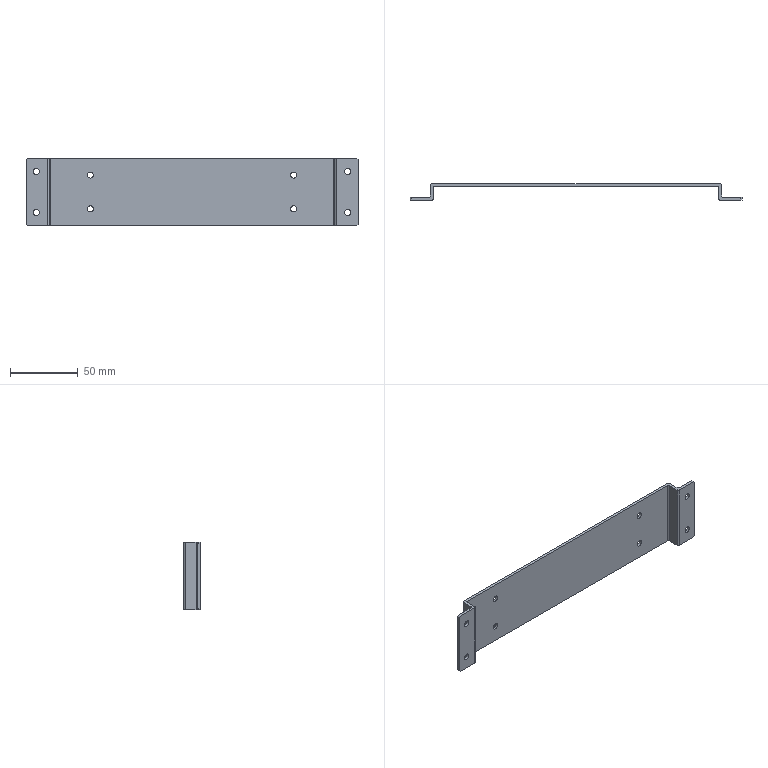Part | NX | 1 solid | 34 faces | box 245 x 12 x 50 mm | volume 26242 mm3 | plane 18 | cylinder 16 | commonest cylinder face diameters 2 x8 4.5 x8
STEP:
#1=CARTESIAN_POINT('',(-41.764,0.,49.));
#2=VERTEX_POINT('',#1);
#3=CARTESIAN_POINT('',(-41.764,0.,1.));
#4=VERTEX_POINT('',#3);
#5=CARTESIAN_POINT('',(-41.764,0.,50.));
#6=DIRECTION('',(0.,0.,-1.));
#7=VECTOR('',#6,1000.);
#8=LINE('',#5,#7);
#9=EDGE_CURVE('',#2,#4,#8,.T.);
#10=ORIENTED_EDGE('',*,*,#9,.T.);
#11=CARTESIAN_POINT('',(-41.764,-2.,1.));
#12=VERTEX_POINT('',#11);
#13=CARTESIAN_POINT('',(-41.764,0.,1.));
#14=DIRECTION('',(0.,-1.,0.));
#15=VECTOR('',#14,1000.);
#16=LINE('',#13,#15);
#17=EDGE_CURVE('',#4,#12,#16,.T.);
#18=ORIENTED_EDGE('',*,*,#17,.T.);
#19=CARTESIAN_POINT('',(-41.764,-2.,49.));
#20=VERTEX_POINT('',#19);
#21=CARTESIAN_POINT('',(-41.764,-2.,50.));
#22=DIRECTION('',(0.,0.,-1.));
#23=VECTOR('',#22,1000.);
#24=LINE('',#21,#23);
#25=EDGE_CURVE('',#20,#12,#24,.T.);
#26=ORIENTED_EDGE('',*,*,#25,.F.);
#27=CARTESIAN_POINT('',(-41.764,0.,49.));
#28=DIRECTION('',(0.,1.,0.));
#29=VECTOR('',#28,1000.);
#30=LINE('',#27,#29);
#31=EDGE_CURVE('',#20,#2,#30,.T.);
#32=ORIENTED_EDGE('',*,*,#31,.T.);
#33=EDGE_LOOP('',(#10,#18,#26,#32));
#34=FACE_BOUND('',#33,.T.);
#35=CARTESIAN_POINT('',(-41.764,0.,50.));
#36=DIRECTION('',(1.,0.,0.));
#37=DIRECTION('',(0.,0.,-1.));
#38=AXIS2_PLACEMENT_3D('',#35,#36,#37);
#39=PLANE('',#38);
#40=ADVANCED_FACE('',(#34),#39,.F.);
#41=CARTESIAN_POINT('',(-34.264,-2.,12.25));
#42=VERTEX_POINT('',#41);
#43=CARTESIAN_POINT('',(-34.264,-2.,10.));
#44=DIRECTION('',(0.,1.,0.));
#45=DIRECTION('',(0.,0.,1.));
#46=AXIS2_PLACEMENT_3D('',#43,#44,#45);
#47=CIRCLE('',#46,2.25);
#48=EDGE_CURVE('',#42,#42,#47,.T.);
#49=ORIENTED_EDGE('',*,*,#48,.T.);
#50=EDGE_LOOP('',(#49));
#51=FACE_BOUND('',#50,.T.);
#52=CARTESIAN_POINT('',(-34.264,-2.,42.25));
#53=VERTEX_POINT('',#52);
#54=CARTESIAN_POINT('',(-34.264,-2.,40.));
#55=DIRECTION('',(0.,1.,0.));
#56=DIRECTION('',(0.,0.,1.));
#57=AXIS2_PLACEMENT_3D('',#54,#55,#56);
#58=CIRCLE('',#57,2.25);
#59=EDGE_CURVE('',#53,#53,#58,.T.);
#60=ORIENTED_EDGE('',*,*,#59,.T.);
#61=EDGE_LOOP('',(#60));
#62=FACE_BOUND('',#61,.T.);
#63=ORIENTED_EDGE('',*,*,#25,.T.);
#64=CARTESIAN_POINT('',(-40.764,-2.,0.));
#65=VERTEX_POINT('',#64);
#66=CARTESIAN_POINT('',(-41.764,-2.,1.));
#67=DIRECTION('',(-0.7071,0.,0.7071));
#68=VECTOR('',#67,1000.);
#69=LINE('',#66,#68);
#70=EDGE_CURVE('',#12,#65,#69,.F.);
#71=ORIENTED_EDGE('',*,*,#70,.T.);
#72=CARTESIAN_POINT('',(-25.764,-2.,0.));
#73=VERTEX_POINT('',#72);
#74=CARTESIAN_POINT('',(-41.764,-2.,0.));
#75=DIRECTION('',(1.,0.,0.));
#76=VECTOR('',#75,1000.);
#77=LINE('',#74,#76);
#78=EDGE_CURVE('',#65,#73,#77,.T.);
#79=ORIENTED_EDGE('',*,*,#78,.T.);
#80=CARTESIAN_POINT('',(-25.764,-2.,50.));
#81=VERTEX_POINT('',#80);
#82=CARTESIAN_POINT('',(-25.764,-2.,50.));
#83=DIRECTION('',(0.,0.,-1.));
#84=VECTOR('',#83,1000.);
#85=LINE('',#82,#84);
#86=EDGE_CURVE('',#81,#73,#85,.T.);
#87=ORIENTED_EDGE('',*,*,#86,.F.);
#88=CARTESIAN_POINT('',(-40.764,-2.,50.));
#89=VERTEX_POINT('',#88);
#90=CARTESIAN_POINT('',(-41.764,-2.,50.));
#91=DIRECTION('',(1.,0.,0.));
#92=VECTOR('',#91,1000.);
#93=LINE('',#90,#92);
#94=EDGE_CURVE('',#89,#81,#93,.T.);
#95=ORIENTED_EDGE('',*,*,#94,.F.);
#96=CARTESIAN_POINT('',(-40.764,-2.,50.));
#97=DIRECTION('',(-0.7071,0.,-0.7071));
#98=VECTOR('',#97,1000.);
#99=LINE('',#96,#98);
#100=EDGE_CURVE('',#89,#20,#99,.T.);
#101=ORIENTED_EDGE('',*,*,#100,.T.);
#102=EDGE_LOOP('',(#63,#71,#79,#87,#95,#101));
#103=FACE_BOUND('',#102,.T.);
#104=CARTESIAN_POINT('',(-41.764,-2.,50.));
#105=DIRECTION('',(0.,1.,0.));
#106=DIRECTION('',(0.,0.,1.));
#107=AXIS2_PLACEMENT_3D('',#104,#105,#106);
#108=PLANE('',#107);
#109=ADVANCED_FACE('',(#51,#62,#103),#108,.F.);
#110=CARTESIAN_POINT('',(-24.764,-1.,0.));
#111=VERTEX_POINT('',#110);
#112=CARTESIAN_POINT('',(-25.764,-1.,0.));
#113=DIRECTION('',(0.,0.,1.));
#114=DIRECTION('',(1.,0.,0.));
#115=AXIS2_PLACEMENT_3D('',#112,#113,#114);
#116=CIRCLE('',#115,1.);
#117=EDGE_CURVE('',#73,#111,#116,.T.);
#118=ORIENTED_EDGE('',*,*,#117,.T.);
#119=CARTESIAN_POINT('',(-24.764,-1.,50.));
#120=VERTEX_POINT('',#119);
#121=CARTESIAN_POINT('',(-24.764,-1.,50.));
#122=DIRECTION('',(0.,0.,-1.));
#123=VECTOR('',#122,1000.);
#124=LINE('',#121,#123);
#125=EDGE_CURVE('',#120,#111,#124,.T.);
#126=ORIENTED_EDGE('',*,*,#125,.F.);
#127=CARTESIAN_POINT('',(-25.764,-1.,50.));
#128=DIRECTION('',(0.,0.,1.));
#129=DIRECTION('',(1.,0.,0.));
#130=AXIS2_PLACEMENT_3D('',#127,#128,#129);
#131=CIRCLE('',#130,1.);
#132=EDGE_CURVE('',#81,#120,#131,.T.);
#133=ORIENTED_EDGE('',*,*,#132,.F.);
#134=ORIENTED_EDGE('',*,*,#86,.T.);
#135=EDGE_LOOP('',(#118,#126,#133,#134));
#136=FACE_BOUND('',#135,.T.);
#137=CARTESIAN_POINT('',(-25.764,-1.,50.));
#138=DIRECTION('',(0.,0.,-1.));
#139=DIRECTION('',(-1.,0.,0.));
#140=AXIS2_PLACEMENT_3D('',#137,#138,#139);
#141=CYLINDRICAL_SURFACE('',#140,1.);
#142=ADVANCED_FACE('',(#136),#141,.T.);
#143=CARTESIAN_POINT('',(-24.764,7.,0.));
#144=VERTEX_POINT('',#143);
#145=CARTESIAN_POINT('',(-24.764,-1.,0.));
#146=DIRECTION('',(0.,1.,0.));
#147=VECTOR('',#146,1000.);
#148=LINE('',#145,#147);
#149=EDGE_CURVE('',#111,#144,#148,.T.);
#150=ORIENTED_EDGE('',*,*,#149,.T.);
#151=CARTESIAN_POINT('',(-24.764,7.,50.));
#152=VERTEX_POINT('',#151);
#153=CARTESIAN_POINT('',(-24.764,7.,50.));
#154=DIRECTION('',(0.,0.,-1.));
#155=VECTOR('',#154,1000.);
#156=LINE('',#153,#155);
#157=EDGE_CURVE('',#152,#144,#156,.T.);
#158=ORIENTED_EDGE('',*,*,#157,.F.);
#159=CARTESIAN_POINT('',(-24.764,-1.,50.));
#160=DIRECTION('',(0.,1.,0.));
#161=VECTOR('',#160,1000.);
#162=LINE('',#159,#161);
#163=EDGE_CURVE('',#120,#152,#162,.T.);
#164=ORIENTED_EDGE('',*,*,#163,.F.);
#165=ORIENTED_EDGE('',*,*,#125,.T.);
#166=EDGE_LOOP('',(#150,#158,#164,#165));
#167=FACE_BOUND('',#166,.T.);
#168=CARTESIAN_POINT('',(-24.764,-1.,50.));
#169=DIRECTION('',(-1.,0.,0.));
#170=DIRECTION('',(0.,0.,1.));
#171=AXIS2_PLACEMENT_3D('',#168,#169,#170);
#172=PLANE('',#171);
#173=ADVANCED_FACE('',(#167),#172,.F.);
#174=CARTESIAN_POINT('',(-23.764,8.,0.));
#175=VERTEX_POINT('',#174);
#176=CARTESIAN_POINT('',(-23.764,7.,0.));
#177=DIRECTION('',(0.,0.,-1.));
#178=DIRECTION('',(-1.,0.,0.));
#179=AXIS2_PLACEMENT_3D('',#176,#177,#178);
#180=CIRCLE('',#179,1.);
#181=EDGE_CURVE('',#144,#175,#180,.T.);
#182=ORIENTED_EDGE('',*,*,#181,.T.);
#183=CARTESIAN_POINT('',(-23.764,8.,50.));
#184=VERTEX_POINT('',#183);
#185=CARTESIAN_POINT('',(-23.764,8.,50.));
#186=DIRECTION('',(0.,0.,-1.));
#187=VECTOR('',#186,1000.);
#188=LINE('',#185,#187);
#189=EDGE_CURVE('',#184,#175,#188,.T.);
#190=ORIENTED_EDGE('',*,*,#189,.F.);
#191=CARTESIAN_POINT('',(-23.764,7.,50.));
#192=DIRECTION('',(0.,0.,-1.));
#193=DIRECTION('',(-1.,0.,0.));
#194=AXIS2_PLACEMENT_3D('',#191,#192,#193);
#195=CIRCLE('',#194,1.);
#196=EDGE_CURVE('',#152,#184,#195,.T.);
#197=ORIENTED_EDGE('',*,*,#196,.F.);
#198=ORIENTED_EDGE('',*,*,#157,.T.);
#199=EDGE_LOOP('',(#182,#190,#197,#198));
#200=FACE_BOUND('',#199,.T.);
#201=CARTESIAN_POINT('',(-23.764,7.,50.));
#202=DIRECTION('',(0.,0.,-1.));
#203=DIRECTION('',(-1.,0.,0.));
#204=AXIS2_PLACEMENT_3D('',#201,#202,#203);
#205=CYLINDRICAL_SURFACE('',#204,1.);
#206=ADVANCED_FACE('',(#200),#205,.F.);
#207=CARTESIAN_POINT('',(153.486,8.,12.5));
#208=VERTEX_POINT('',#207);
#209=CARTESIAN_POINT('',(155.736,8.,12.5));
#210=DIRECTION('',(0.,1.,0.));
#211=DIRECTION('',(-1.,0.,0.));
#212=AXIS2_PLACEMENT_3D('',#209,#210,#211);
#213=CIRCLE('',#212,2.25);
#214=EDGE_CURVE('',#208,#208,#213,.T.);
#215=ORIENTED_EDGE('',*,*,#214,.T.);
#216=EDGE_LOOP('',(#215));
#217=FACE_BOUND('',#216,.T.);
#218=CARTESIAN_POINT('',(3.486,8.,12.5));
#219=VERTEX_POINT('',#218);
#220=CARTESIAN_POINT('',(5.736,8.,12.5));
#221=DIRECTION('',(0.,1.,0.));
#222=DIRECTION('',(-1.,0.,0.));
#223=AXIS2_PLACEMENT_3D('',#220,#221,#222);
#224=CIRCLE('',#223,2.25);
#225=EDGE_CURVE('',#219,#219,#224,.T.);
#226=ORIENTED_EDGE('',*,*,#225,.T.);
#227=EDGE_LOOP('',(#226));
#228=FACE_BOUND('',#227,.T.);
#229=CARTESIAN_POINT('',(3.486,8.,37.5));
#230=VERTEX_POINT('',#229);
#231=CARTESIAN_POINT('',(5.736,8.,37.5));
#232=DIRECTION('',(0.,1.,0.));
#233=DIRECTION('',(-1.,0.,0.));
#234=AXIS2_PLACEMENT_3D('',#231,#232,#233);
#235=CIRCLE('',#234,2.25);
#236=EDGE_CURVE('',#230,#230,#235,.T.);
#237=ORIENTED_EDGE('',*,*,#236,.T.);
#238=EDGE_LOOP('',(#237));
#239=FACE_BOUND('',#238,.T.);
#240=CARTESIAN_POINT('',(153.486,8.,37.5));
#241=VERTEX_POINT('',#240);
#242=CARTESIAN_POINT('',(155.736,8.,37.5));
#243=DIRECTION('',(0.,1.,0.));
#244=DIRECTION('',(-1.,0.,0.));
#245=AXIS2_PLACEMENT_3D('',#242,#243,#244);
#246=CIRCLE('',#245,2.25);
#247=EDGE_CURVE('',#241,#241,#246,.T.);
#248=ORIENTED_EDGE('',*,*,#247,.T.);
#249=EDGE_LOOP('',(#248));
#250=FACE_BOUND('',#249,.T.);
#251=CARTESIAN_POINT('',(185.236,8.,0.));
#252=VERTEX_POINT('',#251);
#253=CARTESIAN_POINT('',(-23.764,8.,0.));
#254=DIRECTION('',(1.,0.,0.));
#255=VECTOR('',#254,1000.);
#256=LINE('',#253,#255);
#257=EDGE_CURVE('',#175,#252,#256,.T.);
#258=ORIENTED_EDGE('',*,*,#257,.T.);
#259=CARTESIAN_POINT('',(185.236,8.,50.));
#260=VERTEX_POINT('',#259);
#261=CARTESIAN_POINT('',(185.236,8.,50.));
#262=DIRECTION('',(0.,0.,-1.));
#263=VECTOR('',#262,1000.);
#264=LINE('',#261,#263);
#265=EDGE_CURVE('',#260,#252,#264,.T.);
#266=ORIENTED_EDGE('',*,*,#265,.F.);
#267=CARTESIAN_POINT('',(-23.764,8.,50.));
#268=DIRECTION('',(1.,0.,0.));
#269=VECTOR('',#268,1000.);
#270=LINE('',#267,#269);
#271=EDGE_CURVE('',#184,#260,#270,.T.);
#272=ORIENTED_EDGE('',*,*,#271,.F.);
#273=ORIENTED_EDGE('',*,*,#189,.T.);
#274=EDGE_LOOP('',(#258,#266,#272,#273));
#275=FACE_BOUND('',#274,.T.);
#276=CARTESIAN_POINT('',(-23.764,8.,50.));
#277=DIRECTION('',(0.,1.,0.));
#278=DIRECTION('',(-1.,0.,0.));
#279=AXIS2_PLACEMENT_3D('',#276,#277,#278);
#280=PLANE('',#279);
#281=ADVANCED_FACE('',(#217,#228,#239,#250,#275),#280,.F.);
#282=CARTESIAN_POINT('',(186.236,7.,0.));
#283=VERTEX_POINT('',#282);
#284=CARTESIAN_POINT('',(185.236,7.,0.));
#285=DIRECTION('',(0.,0.,-1.));
#286=DIRECTION('',(-1.,0.,0.));
#287=AXIS2_PLACEMENT_3D('',#284,#285,#286);
#288=CIRCLE('',#287,1.);
#289=EDGE_CURVE('',#252,#283,#288,.T.);
#290=ORIENTED_EDGE('',*,*,#289,.T.);
#291=CARTESIAN_POINT('',(186.236,7.,50.));
#292=VERTEX_POINT('',#291);
#293=CARTESIAN_POINT('',(186.236,7.,50.));
#294=DIRECTION('',(0.,0.,-1.));
#295=VECTOR('',#294,1000.);
#296=LINE('',#293,#295);
#297=EDGE_CURVE('',#292,#283,#296,.T.);
#298=ORIENTED_EDGE('',*,*,#297,.F.);
#299=CARTESIAN_POINT('',(185.236,7.,50.));
#300=DIRECTION('',(0.,0.,-1.));
#301=DIRECTION('',(-1.,0.,0.));
#302=AXIS2_PLACEMENT_3D('',#299,#300,#301);
#303=CIRCLE('',#302,1.);
#304=EDGE_CURVE('',#260,#292,#303,.T.);
#305=ORIENTED_EDGE('',*,*,#304,.F.);
#306=ORIENTED_EDGE('',*,*,#265,.T.);
#307=EDGE_LOOP('',(#290,#298,#305,#306));
#308=FACE_BOUND('',#307,.T.);
#309=CARTESIAN_POINT('',(185.236,7.,50.));
#310=DIRECTION('',(0.,0.,-1.));
#311=DIRECTION('',(-1.,0.,0.));
#312=AXIS2_PLACEMENT_3D('',#309,#310,#311);
#313=CYLINDRICAL_SURFACE('',#312,1.);
#314=ADVANCED_FACE('',(#308),#313,.F.);
#315=CARTESIAN_POINT('',(186.236,-1.,0.));
#316=VERTEX_POINT('',#315);
#317=CARTESIAN_POINT('',(186.236,7.,0.));
#318=DIRECTION('',(0.,-1.,0.));
#319=VECTOR('',#318,1000.);
#320=LINE('',#317,#319);
#321=EDGE_CURVE('',#283,#316,#320,.T.);
#322=ORIENTED_EDGE('',*,*,#321,.T.);
#323=CARTESIAN_POINT('',(186.236,-1.,50.));
#324=VERTEX_POINT('',#323);
#325=CARTESIAN_POINT('',(186.236,-1.,50.));
#326=DIRECTION('',(0.,0.,-1.));
#327=VECTOR('',#326,1000.);
#328=LINE('',#325,#327);
#329=EDGE_CURVE('',#324,#316,#328,.T.);
#330=ORIENTED_EDGE('',*,*,#329,.F.);
#331=CARTESIAN_POINT('',(186.236,7.,50.));
#332=DIRECTION('',(0.,-1.,0.));
#333=VECTOR('',#332,1000.);
#334=LINE('',#331,#333);
#335=EDGE_CURVE('',#292,#324,#334,.T.);
#336=ORIENTED_EDGE('',*,*,#335,.F.);
#337=ORIENTED_EDGE('',*,*,#297,.T.);
#338=EDGE_LOOP('',(#322,#330,#336,#337));
#339=FACE_BOUND('',#338,.T.);
#340=CARTESIAN_POINT('',(186.236,7.,50.));
#341=DIRECTION('',(1.,0.,0.));
#342=DIRECTION('',(0.,0.,-1.));
#343=AXIS2_PLACEMENT_3D('',#340,#341,#342);
#344=PLANE('',#343);
#345=ADVANCED_FACE('',(#339),#344,.F.);
#346=CARTESIAN_POINT('',(187.236,-2.,0.));
#347=VERTEX_POINT('',#346);
#348=CARTESIAN_POINT('',(187.236,-1.,0.));
#349=DIRECTION('',(0.,0.,1.));
#350=DIRECTION('',(1.,0.,0.));
#351=AXIS2_PLACEMENT_3D('',#348,#349,#350);
#352=CIRCLE('',#351,1.);
#353=EDGE_CURVE('',#316,#347,#352,.T.);
#354=ORIENTED_EDGE('',*,*,#353,.T.);
#355=CARTESIAN_POINT('',(187.236,-2.,50.));
#356=VERTEX_POINT('',#355);
#357=CARTESIAN_POINT('',(187.236,-2.,50.));
#358=DIRECTION('',(0.,0.,-1.));
#359=VECTOR('',#358,1000.);
#360=LINE('',#357,#359);
#361=EDGE_CURVE('',#356,#347,#360,.T.);
#362=ORIENTED_EDGE('',*,*,#361,.F.);
#363=CARTESIAN_POINT('',(187.236,-1.,50.));
#364=DIRECTION('',(0.,0.,1.));
#365=DIRECTION('',(1.,0.,0.));
#366=AXIS2_PLACEMENT_3D('',#363,#364,#365);
#367=CIRCLE('',#366,1.);
#368=EDGE_CURVE('',#324,#356,#367,.T.);
#369=ORIENTED_EDGE('',*,*,#368,.F.);
#370=ORIENTED_EDGE('',*,*,#329,.T.);
#371=EDGE_LOOP('',(#354,#362,#369,#370));
#372=FACE_BOUND('',#371,.T.);
#373=CARTESIAN_POINT('',(187.236,-1.,50.));
#374=DIRECTION('',(0.,0.,-1.));
#375=DIRECTION('',(-1.,0.,0.));
#376=AXIS2_PLACEMENT_3D('',#373,#374,#375);
#377=CYLINDRICAL_SURFACE('',#376,1.);
#378=ADVANCED_FACE('',(#372),#377,.T.);
#379=CARTESIAN_POINT('',(195.736,-2.,42.25));
#380=VERTEX_POINT('',#379);
#381=CARTESIAN_POINT('',(195.736,-2.,40.));
#382=DIRECTION('',(0.,1.,0.));
#383=DIRECTION('',(0.,0.,1.));
#384=AXIS2_PLACEMENT_3D('',#381,#382,#383);
#385=CIRCLE('',#384,2.25);
#386=EDGE_CURVE('',#380,#380,#385,.T.);
#387=ORIENTED_EDGE('',*,*,#386,.T.);
#388=EDGE_LOOP('',(#387));
#389=FACE_BOUND('',#388,.T.);
#390=CARTESIAN_POINT('',(195.736,-2.,12.25));
#391=VERTEX_POINT('',#390);
#392=CARTESIAN_POINT('',(195.736,-2.,10.));
#393=DIRECTION('',(0.,1.,0.));
#394=DIRECTION('',(0.,0.,1.));
#395=AXIS2_PLACEMENT_3D('',#392,#393,#394);
#396=CIRCLE('',#395,2.25);
#397=EDGE_CURVE('',#391,#391,#396,.T.);
#398=ORIENTED_EDGE('',*,*,#397,.T.);
#399=EDGE_LOOP('',(#398));
#400=FACE_BOUND('',#399,.T.);
#401=CARTESIAN_POINT('',(203.236,-2.,49.));
#402=VERTEX_POINT('',#401);
#403=CARTESIAN_POINT('',(203.236,-2.,1.));
#404=VERTEX_POINT('',#403);
#405=CARTESIAN_POINT('',(203.236,-2.,50.));
#406=DIRECTION('',(0.,0.,-1.));
#407=VECTOR('',#406,1000.);
#408=LINE('',#405,#407);
#409=EDGE_CURVE('',#402,#404,#408,.T.);
#410=ORIENTED_EDGE('',*,*,#409,.F.);
#411=CARTESIAN_POINT('',(202.236,-2.,50.));
#412=VERTEX_POINT('',#411);
#413=CARTESIAN_POINT('',(202.236,-2.,50.));
#414=DIRECTION('',(-0.7071,0.,0.7071));
#415=VECTOR('',#414,1000.);
#416=LINE('',#413,#415);
#417=EDGE_CURVE('',#402,#412,#416,.T.);
#418=ORIENTED_EDGE('',*,*,#417,.T.);
#419=CARTESIAN_POINT('',(187.236,-2.,50.));
#420=DIRECTION('',(1.,0.,0.));
#421=VECTOR('',#420,1000.);
#422=LINE('',#419,#421);
#423=EDGE_CURVE('',#356,#412,#422,.T.);
#424=ORIENTED_EDGE('',*,*,#423,.F.);
#425=ORIENTED_EDGE('',*,*,#361,.T.);
#426=CARTESIAN_POINT('',(202.236,-2.,0.));
#427=VERTEX_POINT('',#426);
#428=CARTESIAN_POINT('',(187.236,-2.,0.));
#429=DIRECTION('',(1.,0.,0.));
#430=VECTOR('',#429,1000.);
#431=LINE('',#428,#430);
#432=EDGE_CURVE('',#347,#427,#431,.T.);
#433=ORIENTED_EDGE('',*,*,#432,.T.);
#434=CARTESIAN_POINT('',(203.236,-2.,1.));
#435=DIRECTION('',(-0.7071,0.,-0.7071));
#436=VECTOR('',#435,1000.);
#437=LINE('',#434,#436);
#438=EDGE_CURVE('',#427,#404,#437,.F.);
#439=ORIENTED_EDGE('',*,*,#438,.T.);
#440=EDGE_LOOP('',(#410,#418,#424,#425,#433,#439));
#441=FACE_BOUND('',#440,.T.);
#442=CARTESIAN_POINT('',(187.236,-2.,50.));
#443=DIRECTION('',(0.,1.,0.));
#444=DIRECTION('',(0.,0.,1.));
#445=AXIS2_PLACEMENT_3D('',#442,#443,#444);
#446=PLANE('',#445);
#447=ADVANCED_FACE('',(#389,#400,#441),#446,.F.);
#448=CARTESIAN_POINT('',(203.236,0.,49.));
#449=VERTEX_POINT('',#448);
#450=CARTESIAN_POINT('',(203.236,0.,1.));
#451=VERTEX_POINT('',#450);
#452=CARTESIAN_POINT('',(203.236,0.,50.));
#453=DIRECTION('',(0.,0.,-1.));
#454=VECTOR('',#453,1000.);
#455=LINE('',#452,#454);
#456=EDGE_CURVE('',#449,#451,#455,.T.);
#457=ORIENTED_EDGE('',*,*,#456,.F.);
#458=CARTESIAN_POINT('',(203.236,-2.,49.));
#459=DIRECTION('',(0.,-1.,0.));
#460=VECTOR('',#459,1000.);
#461=LINE('',#458,#460);
#462=EDGE_CURVE('',#449,#402,#461,.T.);
#463=ORIENTED_EDGE('',*,*,#462,.T.);
#464=ORIENTED_EDGE('',*,*,#409,.T.);
#465=CARTESIAN_POINT('',(203.236,-2.,1.));
#466=DIRECTION('',(0.,1.,0.));
#467=VECTOR('',#466,1000.);
#468=LINE('',#465,#467);
#469=EDGE_CURVE('',#404,#451,#468,.T.);
#470=ORIENTED_EDGE('',*,*,#469,.T.);
#471=EDGE_LOOP('',(#457,#463,#464,#470));
#472=FACE_BOUND('',#471,.T.);
#473=CARTESIAN_POINT('',(203.236,-2.,50.));
#474=DIRECTION('',(-1.,0.,0.));
#475=DIRECTION('',(0.,0.,1.));
#476=AXIS2_PLACEMENT_3D('',#473,#474,#475);
#477=PLANE('',#476);
#478=ADVANCED_FACE('',(#472),#477,.F.);
#479=CARTESIAN_POINT('',(195.736,0.,42.25));
#480=VERTEX_POINT('',#479);
#481=CARTESIAN_POINT('',(195.736,0.,40.));
#482=DIRECTION('',(0.,1.,0.));
#483=DIRECTION('',(0.,0.,1.));
#484=AXIS2_PLACEMENT_3D('',#481,#482,#483);
#485=CIRCLE('',#484,2.25);
#486=EDGE_CURVE('',#480,#480,#485,.T.);
#487=ORIENTED_EDGE('',*,*,#486,.F.);
#488=EDGE_LOOP('',(#487));
#489=FACE_BOUND('',#488,.T.);
#490=CARTESIAN_POINT('',(195.736,0.,12.25));
#491=VERTEX_POINT('',#490);
#492=CARTESIAN_POINT('',(195.736,0.,10.));
#493=DIRECTION('',(0.,1.,0.));
#494=DIRECTION('',(0.,0.,1.));
#495=AXIS2_PLACEMENT_3D('',#492,#493,#494);
#496=CIRCLE('',#495,2.25);
#497=EDGE_CURVE('',#491,#491,#496,.T.);
#498=ORIENTED_EDGE('',*,*,#497,.F.);
#499=EDGE_LOOP('',(#498));
#500=FACE_BOUND('',#499,.T.);
#501=CARTESIAN_POINT('',(202.236,0.,50.));
#502=VERTEX_POINT('',#501);
#503=CARTESIAN_POINT('',(189.236,0.,50.));
#504=VERTEX_POINT('',#503);
#505=CARTESIAN_POINT('',(189.236,0.,50.));
#506=DIRECTION('',(-1.,0.,0.));
#507=VECTOR('',#506,1000.);
#508=LINE('',#505,#507);
#509=EDGE_CURVE('',#502,#504,#508,.T.);
#510=ORIENTED_EDGE('',*,*,#509,.F.);
#511=CARTESIAN_POINT('',(202.236,0.,50.));
#512=DIRECTION('',(0.7071,0.,-0.7071));
#513=VECTOR('',#512,1000.);
#514=LINE('',#511,#513);
#515=EDGE_CURVE('',#502,#449,#514,.T.);
#516=ORIENTED_EDGE('',*,*,#515,.T.);
#517=ORIENTED_EDGE('',*,*,#456,.T.);
#518=CARTESIAN_POINT('',(202.236,0.,0.));
#519=VERTEX_POINT('',#518);
#520=CARTESIAN_POINT('',(203.236,0.,1.));
#521=DIRECTION('',(0.7071,0.,0.7071));
#522=VECTOR('',#521,1000.);
#523=LINE('',#520,#522);
#524=EDGE_CURVE('',#451,#519,#523,.F.);
#525=ORIENTED_EDGE('',*,*,#524,.T.);
#526=CARTESIAN_POINT('',(189.236,0.,0.));
#527=VERTEX_POINT('',#526);
#528=CARTESIAN_POINT('',(189.236,0.,0.));
#529=DIRECTION('',(-1.,0.,0.));
#530=VECTOR('',#529,1000.);
#531=LINE('',#528,#530);
#532=EDGE_CURVE('',#519,#527,#531,.T.);
#533=ORIENTED_EDGE('',*,*,#532,.T.);
#534=CARTESIAN_POINT('',(189.236,0.,50.));
#535=DIRECTION('',(0.,0.,-1.));
#536=VECTOR('',#535,1000.);
#537=LINE('',#534,#536);
#538=EDGE_CURVE('',#504,#527,#537,.T.);
#539=ORIENTED_EDGE('',*,*,#538,.F.);
#540=EDGE_LOOP('',(#510,#516,#517,#525,#533,#539));
#541=FACE_BOUND('',#540,.T.);
#542=CARTESIAN_POINT('',(189.236,0.,50.));
#543=DIRECTION('',(0.,-1.,0.));
#544=DIRECTION('',(0.,0.,-1.));
#545=AXIS2_PLACEMENT_3D('',#542,#543,#544);
#546=PLANE('',#545);
#547=ADVANCED_FACE('',(#489,#500,#541),#546,.F.);
#548=CARTESIAN_POINT('',(188.236,1.,0.));
#549=VERTEX_POINT('',#548);
#550=CARTESIAN_POINT('',(189.236,1.,0.));
#551=DIRECTION('',(0.,0.,-1.));
#552=DIRECTION('',(1.,0.,0.));
#553=AXIS2_PLACEMENT_3D('',#550,#551,#552);
#554=CIRCLE('',#553,1.);
#555=EDGE_CURVE('',#527,#549,#554,.T.);
#556=ORIENTED_EDGE('',*,*,#555,.T.);
#557=CARTESIAN_POINT('',(188.236,1.,50.));
#558=VERTEX_POINT('',#557);
#559=CARTESIAN_POINT('',(188.236,1.,50.));
#560=DIRECTION('',(0.,0.,-1.));
#561=VECTOR('',#560,1000.);
#562=LINE('',#559,#561);
#563=EDGE_CURVE('',#558,#549,#562,.T.);
#564=ORIENTED_EDGE('',*,*,#563,.F.);
#565=CARTESIAN_POINT('',(189.236,1.,50.));
#566=DIRECTION('',(0.,0.,-1.));
#567=DIRECTION('',(1.,0.,0.));
#568=AXIS2_PLACEMENT_3D('',#565,#566,#567);
#569=CIRCLE('',#568,1.);
#570=EDGE_CURVE('',#504,#558,#569,.T.);
#571=ORIENTED_EDGE('',*,*,#570,.F.);
#572=ORIENTED_EDGE('',*,*,#538,.T.);
#573=EDGE_LOOP('',(#556,#564,#571,#572));
#574=FACE_BOUND('',#573,.T.);
#575=CARTESIAN_POINT('',(189.236,1.,50.));
#576=DIRECTION('',(0.,0.,-1.));
#577=DIRECTION('',(-1.,0.,0.));
#578=AXIS2_PLACEMENT_3D('',#575,#576,#577);
#579=CYLINDRICAL_SURFACE('',#578,1.);
#580=ADVANCED_FACE('',(#574),#579,.F.);
#581=CARTESIAN_POINT('',(188.236,9.,0.));
#582=VERTEX_POINT('',#581);
#583=CARTESIAN_POINT('',(188.236,9.,0.));
#584=DIRECTION('',(0.,1.,0.));
#585=VECTOR('',#584,1000.);
#586=LINE('',#583,#585);
#587=EDGE_CURVE('',#549,#582,#586,.T.);
#588=ORIENTED_EDGE('',*,*,#587,.T.);
#589=CARTESIAN_POINT('',(188.236,9.,50.));
#590=VERTEX_POINT('',#589);
#591=CARTESIAN_POINT('',(188.236,9.,50.));
#592=DIRECTION('',(0.,0.,-1.));
#593=VECTOR('',#592,1000.);
#594=LINE('',#591,#593);
#595=EDGE_CURVE('',#590,#582,#594,.T.);
#596=ORIENTED_EDGE('',*,*,#595,.F.);
#597=CARTESIAN_POINT('',(188.236,9.,50.));
#598=DIRECTION('',(0.,1.,0.));
#599=VECTOR('',#598,1000.);
#600=LINE('',#597,#599);
#601=EDGE_CURVE('',#558,#590,#600,.T.);
#602=ORIENTED_EDGE('',*,*,#601,.F.);
#603=ORIENTED_EDGE('',*,*,#563,.T.);
#604=EDGE_LOOP('',(#588,#596,#602,#603));
#605=FACE_BOUND('',#604,.T.);
#606=CARTESIAN_POINT('',(188.236,9.,50.));
#607=DIRECTION('',(-1.,0.,0.));
#608=DIRECTION('',(0.,0.,1.));
#609=AXIS2_PLACEMENT_3D('',#606,#607,#608);
#610=PLANE('',#609);
#611=ADVANCED_FACE('',(#605),#610,.F.);
#612=CARTESIAN_POINT('',(187.236,10.,0.));
#613=VERTEX_POINT('',#612);
#614=CARTESIAN_POINT('',(187.236,9.,0.));
#615=DIRECTION('',(0.,0.,1.));
#616=DIRECTION('',(-1.,0.,0.));
#617=AXIS2_PLACEMENT_3D('',#614,#615,#616);
#618=CIRCLE('',#617,1.);
#619=EDGE_CURVE('',#582,#613,#618,.T.);
#620=ORIENTED_EDGE('',*,*,#619,.T.);
#621=CARTESIAN_POINT('',(187.236,10.,50.));
#622=VERTEX_POINT('',#621);
#623=CARTESIAN_POINT('',(187.236,10.,50.));
#624=DIRECTION('',(0.,0.,-1.));
#625=VECTOR('',#624,1000.);
#626=LINE('',#623,#625);
#627=EDGE_CURVE('',#622,#613,#626,.T.);
#628=ORIENTED_EDGE('',*,*,#627,.F.);
#629=CARTESIAN_POINT('',(187.236,9.,50.));
#630=DIRECTION('',(0.,0.,1.));
#631=DIRECTION('',(-1.,0.,0.));
#632=AXIS2_PLACEMENT_3D('',#629,#630,#631);
#633=CIRCLE('',#632,1.);
#634=EDGE_CURVE('',#590,#622,#633,.T.);
#635=ORIENTED_EDGE('',*,*,#634,.F.);
#636=ORIENTED_EDGE('',*,*,#595,.T.);
#637=EDGE_LOOP('',(#620,#628,#635,#636));
#638=FACE_BOUND('',#637,.T.);
#639=CARTESIAN_POINT('',(187.236,9.,50.));
#640=DIRECTION('',(0.,0.,-1.));
#641=DIRECTION('',(-1.,0.,0.));
#642=AXIS2_PLACEMENT_3D('',#639,#640,#641);
#643=CYLINDRICAL_SURFACE('',#642,1.);
#644=ADVANCED_FACE('',(#638),#643,.T.);
#645=CARTESIAN_POINT('',(155.736,10.,14.75));
#646=VERTEX_POINT('',#645);
#647=CARTESIAN_POINT('',(155.736,10.,12.5));
#648=DIRECTION('',(0.,1.,0.));
#649=DIRECTION('',(0.,0.,1.));
#650=AXIS2_PLACEMENT_3D('',#647,#648,#649);
#651=CIRCLE('',#650,2.25);
#652=EDGE_CURVE('',#646,#646,#651,.T.);
#653=ORIENTED_EDGE('',*,*,#652,.F.);
#654=EDGE_LOOP('',(#653));
#655=FACE_BOUND('',#654,.T.);
#656=CARTESIAN_POINT('',(5.736,10.,14.75));
#657=VERTEX_POINT('',#656);
#658=CARTESIAN_POINT('',(5.736,10.,12.5));
#659=DIRECTION('',(0.,1.,0.));
#660=DIRECTION('',(0.,0.,1.));
#661=AXIS2_PLACEMENT_3D('',#658,#659,#660);
#662=CIRCLE('',#661,2.25);
#663=EDGE_CURVE('',#657,#657,#662,.T.);
#664=ORIENTED_EDGE('',*,*,#663,.F.);
#665=EDGE_LOOP('',(#664));
#666=FACE_BOUND('',#665,.T.);
#667=CARTESIAN_POINT('',(5.736,10.,39.75));
#668=VERTEX_POINT('',#667);
#669=CARTESIAN_POINT('',(5.736,10.,37.5));
#670=DIRECTION('',(0.,1.,0.));
#671=DIRECTION('',(0.,0.,1.));
#672=AXIS2_PLACEMENT_3D('',#669,#670,#671);
#673=CIRCLE('',#672,2.25);
#674=EDGE_CURVE('',#668,#668,#673,.T.);
#675=ORIENTED_EDGE('',*,*,#674,.F.);
#676=EDGE_LOOP('',(#675));
#677=FACE_BOUND('',#676,.T.);
#678=CARTESIAN_POINT('',(155.736,10.,39.75));
#679=VERTEX_POINT('',#678);
#680=CARTESIAN_POINT('',(155.736,10.,37.5));
#681=DIRECTION('',(0.,1.,0.));
#682=DIRECTION('',(0.,0.,1.));
#683=AXIS2_PLACEMENT_3D('',#680,#681,#682);
#684=CIRCLE('',#683,2.25);
#685=EDGE_CURVE('',#679,#679,#684,.T.);
#686=ORIENTED_EDGE('',*,*,#685,.F.);
#687=EDGE_LOOP('',(#686));
#688=FACE_BOUND('',#687,.T.);
#689=CARTESIAN_POINT('',(-25.764,10.,0.));
#690=VERTEX_POINT('',#689);
#691=CARTESIAN_POINT('',(-25.764,10.,0.));
#692=DIRECTION('',(-1.,0.,0.));
#693=VECTOR('',#692,1000.);
#694=LINE('',#691,#693);
#695=EDGE_CURVE('',#613,#690,#694,.T.);
#696=ORIENTED_EDGE('',*,*,#695,.T.);
#697=CARTESIAN_POINT('',(-25.764,10.,50.));
#698=VERTEX_POINT('',#697);
#699=CARTESIAN_POINT('',(-25.764,10.,50.));
#700=DIRECTION('',(0.,0.,-1.));
#701=VECTOR('',#700,1000.);
#702=LINE('',#699,#701);
#703=EDGE_CURVE('',#698,#690,#702,.T.);
#704=ORIENTED_EDGE('',*,*,#703,.F.);
#705=CARTESIAN_POINT('',(-25.764,10.,50.));
#706=DIRECTION('',(-1.,0.,0.));
#707=VECTOR('',#706,1000.);
#708=LINE('',#705,#707);
#709=EDGE_CURVE('',#622,#698,#708,.T.);
#710=ORIENTED_EDGE('',*,*,#709,.F.);
#711=ORIENTED_EDGE('',*,*,#627,.T.);
#712=EDGE_LOOP('',(#696,#704,#710,#711));
#713=FACE_BOUND('',#712,.T.);
#714=CARTESIAN_POINT('',(-25.764,10.,50.));
#715=DIRECTION('',(0.,-1.,0.));
#716=DIRECTION('',(0.,0.,-1.));
#717=AXIS2_PLACEMENT_3D('',#714,#715,#716);
#718=PLANE('',#717);
#719=ADVANCED_FACE('',(#655,#666,#677,#688,#713),#718,.F.);
#720=CARTESIAN_POINT('',(-26.764,9.,0.));
#721=VERTEX_POINT('',#720);
#722=CARTESIAN_POINT('',(-25.764,9.,0.));
#723=DIRECTION('',(0.,0.,1.));
#724=DIRECTION('',(-1.,0.,0.));
#725=AXIS2_PLACEMENT_3D('',#722,#723,#724);
#726=CIRCLE('',#725,1.);
#727=EDGE_CURVE('',#690,#721,#726,.T.);
#728=ORIENTED_EDGE('',*,*,#727,.T.);
#729=CARTESIAN_POINT('',(-26.764,9.,50.));
#730=VERTEX_POINT('',#729);
#731=CARTESIAN_POINT('',(-26.764,9.,50.));
#732=DIRECTION('',(0.,0.,-1.));
#733=VECTOR('',#732,1000.);
#734=LINE('',#731,#733);
#735=EDGE_CURVE('',#730,#721,#734,.T.);
#736=ORIENTED_EDGE('',*,*,#735,.F.);
#737=CARTESIAN_POINT('',(-25.764,9.,50.));
#738=DIRECTION('',(0.,0.,1.));
#739=DIRECTION('',(-1.,0.,0.));
#740=AXIS2_PLACEMENT_3D('',#737,#738,#739);
#741=CIRCLE('',#740,1.);
#742=EDGE_CURVE('',#698,#730,#741,.T.);
#743=ORIENTED_EDGE('',*,*,#742,.F.);
#744=ORIENTED_EDGE('',*,*,#703,.T.);
#745=EDGE_LOOP('',(#728,#736,#743,#744));
#746=FACE_BOUND('',#745,.T.);
#747=CARTESIAN_POINT('',(-25.764,9.,50.));
#748=DIRECTION('',(0.,0.,-1.));
#749=DIRECTION('',(-1.,0.,0.));
#750=AXIS2_PLACEMENT_3D('',#747,#748,#749);
#751=CYLINDRICAL_SURFACE('',#750,1.);
#752=ADVANCED_FACE('',(#746),#751,.T.);
#753=CARTESIAN_POINT('',(-26.764,1.,0.));
#754=VERTEX_POINT('',#753);
#755=CARTESIAN_POINT('',(-26.764,1.,0.));
#756=DIRECTION('',(0.,-1.,0.));
#757=VECTOR('',#756,1000.);
#758=LINE('',#755,#757);
#759=EDGE_CURVE('',#721,#754,#758,.T.);
#760=ORIENTED_EDGE('',*,*,#759,.T.);
#761=CARTESIAN_POINT('',(-26.764,1.,50.));
#762=VERTEX_POINT('',#761);
#763=CARTESIAN_POINT('',(-26.764,1.,50.));
#764=DIRECTION('',(0.,0.,-1.));
#765=VECTOR('',#764,1000.);
#766=LINE('',#763,#765);
#767=EDGE_CURVE('',#762,#754,#766,.T.);
#768=ORIENTED_EDGE('',*,*,#767,.F.);
#769=CARTESIAN_POINT('',(-26.764,1.,50.));
#770=DIRECTION('',(0.,-1.,0.));
#771=VECTOR('',#770,1000.);
#772=LINE('',#769,#771);
#773=EDGE_CURVE('',#730,#762,#772,.T.);
#774=ORIENTED_EDGE('',*,*,#773,.F.);
#775=ORIENTED_EDGE('',*,*,#735,.T.);
#776=EDGE_LOOP('',(#760,#768,#774,#775));
#777=FACE_BOUND('',#776,.T.);
#778=CARTESIAN_POINT('',(-26.764,1.,50.));
#779=DIRECTION('',(1.,0.,0.));
#780=DIRECTION('',(0.,0.,-1.));
#781=AXIS2_PLACEMENT_3D('',#778,#779,#780);
#782=PLANE('',#781);
#783=ADVANCED_FACE('',(#777),#782,.F.);
#784=CARTESIAN_POINT('',(-27.764,0.,0.));
#785=VERTEX_POINT('',#784);
#786=CARTESIAN_POINT('',(-27.764,1.,0.));
#787=DIRECTION('',(0.,0.,-1.));
#788=DIRECTION('',(1.,0.,0.));
#789=AXIS2_PLACEMENT_3D('',#786,#787,#788);
#790=CIRCLE('',#789,1.);
#791=EDGE_CURVE('',#754,#785,#790,.T.);
#792=ORIENTED_EDGE('',*,*,#791,.T.);
#793=CARTESIAN_POINT('',(-27.764,0.,50.));
#794=VERTEX_POINT('',#793);
#795=CARTESIAN_POINT('',(-27.764,0.,50.));
#796=DIRECTION('',(0.,0.,-1.));
#797=VECTOR('',#796,1000.);
#798=LINE('',#795,#797);
#799=EDGE_CURVE('',#794,#785,#798,.T.);
#800=ORIENTED_EDGE('',*,*,#799,.F.);
#801=CARTESIAN_POINT('',(-27.764,1.,50.));
#802=DIRECTION('',(0.,0.,-1.));
#803=DIRECTION('',(1.,0.,0.));
#804=AXIS2_PLACEMENT_3D('',#801,#802,#803);
#805=CIRCLE('',#804,1.);
#806=EDGE_CURVE('',#762,#794,#805,.T.);
#807=ORIENTED_EDGE('',*,*,#806,.F.);
#808=ORIENTED_EDGE('',*,*,#767,.T.);
#809=EDGE_LOOP('',(#792,#800,#807,#808));
#810=FACE_BOUND('',#809,.T.);
#811=CARTESIAN_POINT('',(-27.764,1.,50.));
#812=DIRECTION('',(0.,0.,-1.));
#813=DIRECTION('',(-1.,0.,0.));
#814=AXIS2_PLACEMENT_3D('',#811,#812,#813);
#815=CYLINDRICAL_SURFACE('',#814,1.);
#816=ADVANCED_FACE('',(#810),#815,.F.);
#817=CARTESIAN_POINT('',(-34.264,0.,12.25));
#818=VERTEX_POINT('',#817);
#819=CARTESIAN_POINT('',(-34.264,0.,10.));
#820=DIRECTION('',(0.,1.,0.));
#821=DIRECTION('',(0.,0.,1.));
#822=AXIS2_PLACEMENT_3D('',#819,#820,#821);
#823=CIRCLE('',#822,2.25);
#824=EDGE_CURVE('',#818,#818,#823,.T.);
#825=ORIENTED_EDGE('',*,*,#824,.F.);
#826=EDGE_LOOP('',(#825));
#827=FACE_BOUND('',#826,.T.);
#828=CARTESIAN_POINT('',(-34.264,0.,42.25));
#829=VERTEX_POINT('',#828);
#830=CARTESIAN_POINT('',(-34.264,0.,40.));
#831=DIRECTION('',(0.,1.,0.));
#832=DIRECTION('',(0.,0.,1.));
#833=AXIS2_PLACEMENT_3D('',#830,#831,#832);
#834=CIRCLE('',#833,2.25);
#835=EDGE_CURVE('',#829,#829,#834,.T.);
#836=ORIENTED_EDGE('',*,*,#835,.F.);
#837=EDGE_LOOP('',(#836));
#838=FACE_BOUND('',#837,.T.);
#839=CARTESIAN_POINT('',(-40.764,0.,0.));
#840=VERTEX_POINT('',#839);
#841=CARTESIAN_POINT('',(-41.764,0.,0.));
#842=DIRECTION('',(-1.,0.,0.));
#843=VECTOR('',#842,1000.);
#844=LINE('',#841,#843);
#845=EDGE_CURVE('',#785,#840,#844,.T.);
#846=ORIENTED_EDGE('',*,*,#845,.T.);
#847=CARTESIAN_POINT('',(-41.764,0.,1.));
#848=DIRECTION('',(0.7071,0.,-0.7071));
#849=VECTOR('',#848,1000.);
#850=LINE('',#847,#849);
#851=EDGE_CURVE('',#840,#4,#850,.F.);
#852=ORIENTED_EDGE('',*,*,#851,.T.);
#853=ORIENTED_EDGE('',*,*,#9,.F.);
#854=CARTESIAN_POINT('',(-40.764,0.,50.));
#855=VERTEX_POINT('',#854);
#856=CARTESIAN_POINT('',(-40.764,0.,50.));
#857=DIRECTION('',(0.7071,0.,0.7071));
#858=VECTOR('',#857,1000.);
#859=LINE('',#856,#858);
#860=EDGE_CURVE('',#2,#855,#859,.T.);
#861=ORIENTED_EDGE('',*,*,#860,.T.);
#862=CARTESIAN_POINT('',(-41.764,0.,50.));
#863=DIRECTION('',(-1.,0.,0.));
#864=VECTOR('',#863,1000.);
#865=LINE('',#862,#864);
#866=EDGE_CURVE('',#794,#855,#865,.T.);
#867=ORIENTED_EDGE('',*,*,#866,.F.);
#868=ORIENTED_EDGE('',*,*,#799,.T.);
#869=EDGE_LOOP('',(#846,#852,#853,#861,#867,#868));
#870=FACE_BOUND('',#869,.T.);
#871=CARTESIAN_POINT('',(-41.764,0.,50.));
#872=DIRECTION('',(0.,-1.,0.));
#873=DIRECTION('',(0.,0.,-1.));
#874=AXIS2_PLACEMENT_3D('',#871,#872,#873);
#875=PLANE('',#874);
#876=ADVANCED_FACE('',(#827,#838,#870),#875,.F.);
#877=ORIENTED_EDGE('',*,*,#423,.T.);
#878=CARTESIAN_POINT('',(202.236,0.,50.));
#879=DIRECTION('',(0.,1.,0.));
#880=VECTOR('',#879,1000.);
#881=LINE('',#878,#880);
#882=EDGE_CURVE('',#412,#502,#881,.T.);
#883=ORIENTED_EDGE('',*,*,#882,.T.);
#884=ORIENTED_EDGE('',*,*,#509,.T.);
#885=ORIENTED_EDGE('',*,*,#570,.T.);
#886=ORIENTED_EDGE('',*,*,#601,.T.);
#887=ORIENTED_EDGE('',*,*,#634,.T.);
#888=ORIENTED_EDGE('',*,*,#709,.T.);
#889=ORIENTED_EDGE('',*,*,#742,.T.);
#890=ORIENTED_EDGE('',*,*,#773,.T.);
#891=ORIENTED_EDGE('',*,*,#806,.T.);
#892=ORIENTED_EDGE('',*,*,#866,.T.);
#893=CARTESIAN_POINT('',(-40.764,-2.,50.));
#894=DIRECTION('',(0.,-1.,0.));
#895=VECTOR('',#894,1000.);
#896=LINE('',#893,#895);
#897=EDGE_CURVE('',#855,#89,#896,.T.);
#898=ORIENTED_EDGE('',*,*,#897,.T.);
#899=ORIENTED_EDGE('',*,*,#94,.T.);
#900=ORIENTED_EDGE('',*,*,#132,.T.);
#901=ORIENTED_EDGE('',*,*,#163,.T.);
#902=ORIENTED_EDGE('',*,*,#196,.T.);
#903=ORIENTED_EDGE('',*,*,#271,.T.);
#904=ORIENTED_EDGE('',*,*,#304,.T.);
#905=ORIENTED_EDGE('',*,*,#335,.T.);
#906=ORIENTED_EDGE('',*,*,#368,.T.);
#907=EDGE_LOOP('',(#877,#883,#884,#885,#886,#887,#888,#889,#890,#891,#892,#898,#899,#900,#901,#902,#903,#904,#905,#906));
#908=FACE_BOUND('',#907,.T.);
#909=CARTESIAN_POINT('',(-25.764,-1.,50.));
#910=DIRECTION('',(0.,0.,1.));
#911=DIRECTION('',(1.,0.,0.));
#912=AXIS2_PLACEMENT_3D('',#909,#910,#911);
#913=PLANE('',#912);
#914=ADVANCED_FACE('',(#908),#913,.T.);
#915=ORIENTED_EDGE('',*,*,#532,.F.);
#916=CARTESIAN_POINT('',(202.236,-1.,0.));
#917=DIRECTION('',(0.,-1.,0.));
#918=VECTOR('',#917,1000.);
#919=LINE('',#916,#918);
#920=EDGE_CURVE('',#519,#427,#919,.T.);
#921=ORIENTED_EDGE('',*,*,#920,.T.);
#922=ORIENTED_EDGE('',*,*,#432,.F.);
#923=ORIENTED_EDGE('',*,*,#353,.F.);
#924=ORIENTED_EDGE('',*,*,#321,.F.);
#925=ORIENTED_EDGE('',*,*,#289,.F.);
#926=ORIENTED_EDGE('',*,*,#257,.F.);
#927=ORIENTED_EDGE('',*,*,#181,.F.);
#928=ORIENTED_EDGE('',*,*,#149,.F.);
#929=ORIENTED_EDGE('',*,*,#117,.F.);
#930=ORIENTED_EDGE('',*,*,#78,.F.);
#931=CARTESIAN_POINT('',(-40.764,-1.,0.));
#932=DIRECTION('',(0.,1.,0.));
#933=VECTOR('',#932,1000.);
#934=LINE('',#931,#933);
#935=EDGE_CURVE('',#65,#840,#934,.T.);
#936=ORIENTED_EDGE('',*,*,#935,.T.);
#937=ORIENTED_EDGE('',*,*,#845,.F.);
#938=ORIENTED_EDGE('',*,*,#791,.F.);
#939=ORIENTED_EDGE('',*,*,#759,.F.);
#940=ORIENTED_EDGE('',*,*,#727,.F.);
#941=ORIENTED_EDGE('',*,*,#695,.F.);
#942=ORIENTED_EDGE('',*,*,#619,.F.);
#943=ORIENTED_EDGE('',*,*,#587,.F.);
#944=ORIENTED_EDGE('',*,*,#555,.F.);
#945=EDGE_LOOP('',(#915,#921,#922,#923,#924,#925,#926,#927,#928,#929,#930,#936,#937,#938,#939,#940,#941,#942,#943,#944));
#946=FACE_BOUND('',#945,.T.);
#947=CARTESIAN_POINT('',(-25.764,-1.,0.));
#948=DIRECTION('',(0.,0.,1.));
#949=DIRECTION('',(1.,0.,0.));
#950=AXIS2_PLACEMENT_3D('',#947,#948,#949);
#951=PLANE('',#950);
#952=ADVANCED_FACE('',(#946),#951,.F.);
#953=ORIENTED_EDGE('',*,*,#397,.F.);
#954=EDGE_LOOP('',(#953));
#955=FACE_BOUND('',#954,.T.);
#956=ORIENTED_EDGE('',*,*,#497,.T.);
#957=EDGE_LOOP('',(#956));
#958=FACE_BOUND('',#957,.T.);
#959=CARTESIAN_POINT('',(195.736,0.,10.));
#960=DIRECTION('',(0.,1.,0.));
#961=DIRECTION('',(0.,0.,1.));
#962=AXIS2_PLACEMENT_3D('',#959,#960,#961);
#963=CYLINDRICAL_SURFACE('',#962,2.25);
#964=ADVANCED_FACE('',(#955,#958),#963,.F.);
#965=ORIENTED_EDGE('',*,*,#386,.F.);
#966=EDGE_LOOP('',(#965));
#967=FACE_BOUND('',#966,.T.);
#968=ORIENTED_EDGE('',*,*,#486,.T.);
#969=EDGE_LOOP('',(#968));
#970=FACE_BOUND('',#969,.T.);
#971=CARTESIAN_POINT('',(195.736,0.,40.));
#972=DIRECTION('',(0.,1.,0.));
#973=DIRECTION('',(0.,0.,1.));
#974=AXIS2_PLACEMENT_3D('',#971,#972,#973);
#975=CYLINDRICAL_SURFACE('',#974,2.25);
#976=ADVANCED_FACE('',(#967,#970),#975,.F.);
#977=ORIENTED_EDGE('',*,*,#59,.F.);
#978=EDGE_LOOP('',(#977));
#979=FACE_BOUND('',#978,.T.);
#980=ORIENTED_EDGE('',*,*,#835,.T.);
#981=EDGE_LOOP('',(#980));
#982=FACE_BOUND('',#981,.T.);
#983=CARTESIAN_POINT('',(-34.264,0.,40.));
#984=DIRECTION('',(0.,1.,0.));
#985=DIRECTION('',(0.,0.,1.));
#986=AXIS2_PLACEMENT_3D('',#983,#984,#985);
#987=CYLINDRICAL_SURFACE('',#986,2.25);
#988=ADVANCED_FACE('',(#979,#982),#987,.F.);
#989=ORIENTED_EDGE('',*,*,#48,.F.);
#990=EDGE_LOOP('',(#989));
#991=FACE_BOUND('',#990,.T.);
#992=ORIENTED_EDGE('',*,*,#824,.T.);
#993=EDGE_LOOP('',(#992));
#994=FACE_BOUND('',#993,.T.);
#995=CARTESIAN_POINT('',(-34.264,0.,10.));
#996=DIRECTION('',(0.,1.,0.));
#997=DIRECTION('',(0.,0.,1.));
#998=AXIS2_PLACEMENT_3D('',#995,#996,#997);
#999=CYLINDRICAL_SURFACE('',#998,2.25);
#1000=ADVANCED_FACE('',(#991,#994),#999,.F.);
#1001=ORIENTED_EDGE('',*,*,#685,.T.);
#1002=EDGE_LOOP('',(#1001));
#1003=FACE_BOUND('',#1002,.T.);
#1004=ORIENTED_EDGE('',*,*,#247,.F.);
#1005=EDGE_LOOP('',(#1004));
#1006=FACE_BOUND('',#1005,.T.);
#1007=CARTESIAN_POINT('',(155.736,10.,37.5));
#1008=DIRECTION('',(0.,1.,0.));
#1009=DIRECTION('',(0.,0.,1.));
#1010=AXIS2_PLACEMENT_3D('',#1007,#1008,#1009);
#1011=CYLINDRICAL_SURFACE('',#1010,2.25);
#1012=ADVANCED_FACE('',(#1003,#1006),#1011,.F.);
#1013=ORIENTED_EDGE('',*,*,#674,.T.);
#1014=EDGE_LOOP('',(#1013));
#1015=FACE_BOUND('',#1014,.T.);
#1016=ORIENTED_EDGE('',*,*,#236,.F.);
#1017=EDGE_LOOP('',(#1016));
#1018=FACE_BOUND('',#1017,.T.);
#1019=CARTESIAN_POINT('',(5.736,10.,37.5));
#1020=DIRECTION('',(0.,1.,0.));
#1021=DIRECTION('',(0.,0.,1.));
#1022=AXIS2_PLACEMENT_3D('',#1019,#1020,#1021);
#1023=CYLINDRICAL_SURFACE('',#1022,2.25);
#1024=ADVANCED_FACE('',(#1015,#1018),#1023,.F.);
#1025=ORIENTED_EDGE('',*,*,#663,.T.);
#1026=EDGE_LOOP('',(#1025));
#1027=FACE_BOUND('',#1026,.T.);
#1028=ORIENTED_EDGE('',*,*,#225,.F.);
#1029=EDGE_LOOP('',(#1028));
#1030=FACE_BOUND('',#1029,.T.);
#1031=CARTESIAN_POINT('',(5.736,10.,12.5));
#1032=DIRECTION('',(0.,1.,0.));
#1033=DIRECTION('',(0.,0.,1.));
#1034=AXIS2_PLACEMENT_3D('',#1031,#1032,#1033);
#1035=CYLINDRICAL_SURFACE('',#1034,2.25);
#1036=ADVANCED_FACE('',(#1027,#1030),#1035,.F.);
#1037=ORIENTED_EDGE('',*,*,#652,.T.);
#1038=EDGE_LOOP('',(#1037));
#1039=FACE_BOUND('',#1038,.T.);
#1040=ORIENTED_EDGE('',*,*,#214,.F.);
#1041=EDGE_LOOP('',(#1040));
#1042=FACE_BOUND('',#1041,.T.);
#1043=CARTESIAN_POINT('',(155.736,10.,12.5));
#1044=DIRECTION('',(0.,1.,0.));
#1045=DIRECTION('',(0.,0.,1.));
#1046=AXIS2_PLACEMENT_3D('',#1043,#1044,#1045);
#1047=CYLINDRICAL_SURFACE('',#1046,2.25);
#1048=ADVANCED_FACE('',(#1039,#1042),#1047,.F.);
#1049=ORIENTED_EDGE('',*,*,#417,.F.);
#1050=ORIENTED_EDGE('',*,*,#462,.F.);
#1051=ORIENTED_EDGE('',*,*,#515,.F.);
#1052=ORIENTED_EDGE('',*,*,#882,.F.);
#1053=EDGE_LOOP('',(#1049,#1050,#1051,#1052));
#1054=FACE_BOUND('',#1053,.T.);
#1055=CARTESIAN_POINT('',(202.236,-1.,50.));
#1056=DIRECTION('',(0.7071,0.,0.7071));
#1057=DIRECTION('',(0.,-1.,0.));
#1058=AXIS2_PLACEMENT_3D('',#1055,#1056,#1057);
#1059=PLANE('',#1058);
#1060=ADVANCED_FACE('',(#1054),#1059,.T.);
#1061=ORIENTED_EDGE('',*,*,#438,.F.);
#1062=ORIENTED_EDGE('',*,*,#920,.F.);
#1063=ORIENTED_EDGE('',*,*,#524,.F.);
#1064=ORIENTED_EDGE('',*,*,#469,.F.);
#1065=EDGE_LOOP('',(#1061,#1062,#1063,#1064));
#1066=FACE_BOUND('',#1065,.T.);
#1067=CARTESIAN_POINT('',(203.236,-2.,1.));
#1068=DIRECTION('',(-0.7071,0.,0.7071));
#1069=DIRECTION('',(0.,1.,0.));
#1070=AXIS2_PLACEMENT_3D('',#1067,#1068,#1069);
#1071=PLANE('',#1070);
#1072=ADVANCED_FACE('',(#1066),#1071,.F.);
#1073=ORIENTED_EDGE('',*,*,#851,.F.);
#1074=ORIENTED_EDGE('',*,*,#935,.F.);
#1075=ORIENTED_EDGE('',*,*,#70,.F.);
#1076=ORIENTED_EDGE('',*,*,#17,.F.);
#1077=EDGE_LOOP('',(#1073,#1074,#1075,#1076));
#1078=FACE_BOUND('',#1077,.T.);
#1079=CARTESIAN_POINT('',(-41.764,0.,1.));
#1080=DIRECTION('',(0.7071,0.,0.7071));
#1081=DIRECTION('',(0.,-1.,0.));
#1082=AXIS2_PLACEMENT_3D('',#1079,#1080,#1081);
#1083=PLANE('',#1082);
#1084=ADVANCED_FACE('',(#1078),#1083,.F.);
#1085=ORIENTED_EDGE('',*,*,#860,.F.);
#1086=ORIENTED_EDGE('',*,*,#31,.F.);
#1087=ORIENTED_EDGE('',*,*,#100,.F.);
#1088=ORIENTED_EDGE('',*,*,#897,.F.);
#1089=EDGE_LOOP('',(#1085,#1086,#1087,#1088));
#1090=FACE_BOUND('',#1089,.T.);
#1091=CARTESIAN_POINT('',(-40.764,-1.,50.));
#1092=DIRECTION('',(-0.7071,0.,0.7071));
#1093=DIRECTION('',(0.,1.,0.));
#1094=AXIS2_PLACEMENT_3D('',#1091,#1092,#1093);
#1095=PLANE('',#1094);
#1096=ADVANCED_FACE('',(#1090),#1095,.T.);
#1097=CLOSED_SHELL('',(#40,#109,#142,#173,#206,#281,#314,#345,#378,#447,#478,#547,#580,#611,#644,#719,#752,#783,#816,#876,#914,#952,#964,#976,#988,#1000,#1012,#1024,#1036,#1048,#1060,#1072,#1084,#1096));
#1098=MANIFOLD_SOLID_BREP('',#1097);
#1099=(LENGTH_UNIT()NAMED_UNIT(*)SI_UNIT(.MILLI.,.METRE.));
#1100=UNCERTAINTY_MEASURE_WITH_UNIT(LENGTH_MEASURE(0.00001),#1099,'','');
#1101=(NAMED_UNIT(*)PLANE_ANGLE_UNIT()SI_UNIT($,.RADIAN.));
#1102=(NAMED_UNIT(*)SI_UNIT($,.STERADIAN.)SOLID_ANGLE_UNIT());
#1103=(GEOMETRIC_REPRESENTATION_CONTEXT(3)GLOBAL_UNCERTAINTY_ASSIGNED_CONTEXT((#1100))GLOBAL_UNIT_ASSIGNED_CONTEXT((#1099,#1101,#1102))REPRESENTATION_CONTEXT('',''));
#1104=ADVANCED_BREP_SHAPE_REPRESENTATION('',(#1098),#1103);